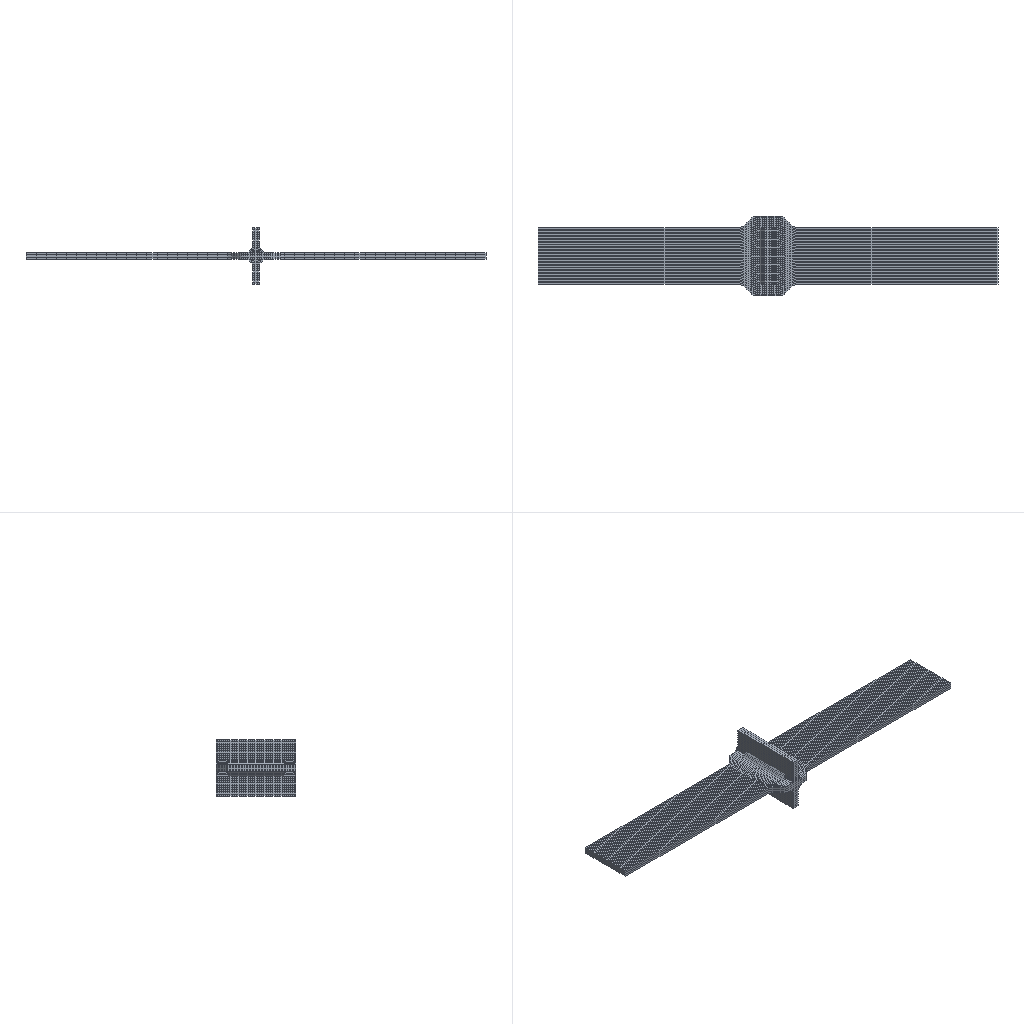Simulation study | abaqus
Set-up summary:
category,name,step,type,value,unit,region
solver,abaqus
solver,version,,,Abaqus/Standard 3DEXPERIENCE R2017x
units,not stated in the deck,,not stated
analysis,deck,,coupled temperature-displacement,coupled temperature-displacement
load_step,Step-del,Step-del,coupled temperature-displacement
load_step,Step-add,Step-add,coupled temperature-displacement
load_step,requested,,,2
mesh,nodes,,,15296
mesh,elements,,,11153
element_type,C3D8RT,,solid,11153
load,load commands in deck,,count,3
bc,support commands in deck,,count,3
material,MATERIAL-1,,in results
check,setup vs results,,match,"per instance, exact: element labels, types and connectivity; labels of the nodes the elements use; coordinates of those nodes at SINGLE_PRECISION in 1 of 2 instance(s)"
Abaqus input file, long lists of numbers shortened:
*Heading
** Job name: Job-2 Model name: Model-1-Copy
** Generated by: Abaqus/CAE 2017
*Preprint, echo=NO, model=NO, history=NO, contact=NO
**
** PARTS
**
*Part, name=Part-1
*Node
      1,  -10.243,          70.,           6.
      2,  -10.243,          70.,           0.
** (14566 more lines like these left out)
*Element, type=C3D8RT
1,  134, 1857,  129,    1,  135, 1859,  136,    6
2, 1857, 1858,  130,  129, 1859, 1860,  137,  136
** (10676 more lines like these left out)
*Nset, nset=Set-5, generate
     1,  14568,      1
*Elset, elset=Set-5, generate
     1,  10678,      1
** Section: Section-1
*Solid Section, elset=Set-5, material=Material-1
,
*End Part
**
*Part, name=add
*Node
      1,   4.243,          60.,           6.
      2,   4.243,          10.,           6.
** (726 more lines like these left out)
*Element, type=C3D8RT
  1, 273, 276,  96,  95, 441, 444, 299, 300
  2, 276, 275,  97,  96, 444, 443, 298, 299
** (473 more lines like these left out)
*Nset, nset=Set-5, generate
   1,  728,    1
*Elset, elset=Set-5, generate
   1,  475,    1
** Section: Section-1
*Solid Section, elset=Set-5, material=Material-1
,
*End Part
**
**
** ASSEMBLY
**
*Assembly, name=Assembly
**
*Instance, name=Part-1-1, part=Part-1
    -2.121,         -10.,     -8.121
*End Instance
**
*Instance, name=add-1, part=add
    -2.121,         -10.,     -8.121
*End Instance
**
*Nset, nset=Set-1, instance=Part-1-1
    13,    14,    15,    16,    33,    34,    44,    45,    49,    50,    54,    55,    65,    70,    71,    76
    82,    91,   213,   214,   215,   216,   217,   218,   219,   220,   221,   222,   223,   224,   225,   226
** (52 more lines like these left out)
*Elset, elset=Set-1, instance=Part-1-1, generate
 10213,  10637,      1
*Nset, nset=Set-4, instance=Part-1-1
    99,   100,   103,   104,   109,   110,   111,   112,   115,   116,   119,   120,   125,   126,   127,   128
  1024,  1025,  1026,  1027,  1028,  1029,  1030,  1031,  1032,  1033,  1034,  1035,  1036,  1037,  1038,  1039
** (397 more lines like these left out)
*Elset, elset=Set-4, instance=Part-1-1
 4108, 4109, 4110, 4111, 4112, 4113, 4114, 4115, 4116, 4117, 4118, 4119, 4120, 4121, 4122, 4123
 4124, 4125, 4126, 4127, 4128, 4129, 4130, 4131, 4132, 4133, 4134, 4135, 4136, 4137, 4138, 4139
** (276 more lines like these left out)
*Nset, nset=Set-5, instance=Part-1-1, generate
     1,  14568,      1
*Elset, elset=Set-5, instance=Part-1-1, generate
     1,  10678,      1
*Nset, nset=Set-6, instance=add-1, generate
   1,  728,    1
*Elset, elset=Set-6, instance=add-1, generate
   1,  475,    1
*Nset, nset=Set-7, instance=Part-1-1, generate
     1,  14568,      1
*Nset, nset=Set-7, instance=add-1, generate
   1,  728,    1
*Elset, elset=Set-7, instance=Part-1-1, generate
     1,  10678,      1
*Elset, elset=Set-7, instance=add-1, generate
   1,  475,    1
*Nset, nset=Set-8, instance=Part-1-1
    13,    14,    15,    16,    33,    34,    44,    45,    49,    50,    54,    55,    65,    70,    71,    76
    82,    91,   213,   214,   215,   216,   217,   218,   219,   220,   221,   222,   223,   224,   225,   226
** (52 more lines like these left out)
*Nset, nset=Set-8, instance=add-1, generate
   1,  728,    1
*Elset, elset=Set-8, instance=Part-1-1, generate
 10213,  10637,      1
*Elset, elset=Set-8, instance=add-1, generate
   1,  475,    1
*Nset, nset=Set-9, instance=add-1, generate
   1,  728,    1
*Elset, elset=Set-9, instance=add-1, generate
   1,  475,    1
*Nset, nset=Set-10, instance=Part-1-1, generate
     1,  14568,      1
*Nset, nset=Set-10, instance=add-1, generate
   1,  728,    1
*Elset, elset=Set-10, instance=Part-1-1, generate
     1,  10678,      1
*Elset, elset=Set-10, instance=add-1, generate
   1,  475,    1
*Elset, elset=_Surf-1_S4, internal, instance=Part-1-1
     3,     6,     9,    12,    15,    18,    21,    24,    27,    30,    33,    36,    39,    42,    45,    48
    51,    54,    57,    60,    63,    66,    69,    72,    75,    78,    81,    84,    87,    90,    93,    96
** (63 more lines like these left out)
*Elset, elset=_Surf-1_S6, internal, instance=Part-1-1
     1,     4,     7,    10,    13,    16,    19,    22,    25,    28,    31,    34,    37,    40,    43,    46
    49,    52,    55,    58,    61,    64,    67,    70,    73,    76,    79,    82,    85,    88,    91,    94
** (50 more lines like these left out)
*Elset, elset=_Surf-1_S3, internal, instance=Part-1-1
  445,  446,  447,  556,  557,  558,  667,  668,  669,  781,  784,  787,  790,  793,  871,  874
  877,  880,  883,  892,  895,  898,  901,  904,  982,  985,  988,  991,  994, 1003, 1006, 1009
** (38 more lines like these left out)
*Elset, elset=_Surf-1_S5, internal, instance=Part-1-1
   553,   554,   555,   664,   665,   666,   775,   776,   777,   783,   786,   789,   792,   795,   873,   876
   879,   882,   885,   894,   897,   900,   903,   906,   984,   987,   990,   993,   996,  1005,  1008,  1011
** (31 more lines like these left out)
*Elset, elset=_Surf-1_S1, internal, instance=Part-1-1
     1,     2,     3,     4,     5,     6,   223,   224,   225,   226,   227,   228,  3553,  3554,  3555,  3556
  3557,  3558,  3559,  3560,  3561,  3562,  3563,  3564,  3565,  3566,  3567,  3568,  3569,  3570,  3571,  3572
** (133 more lines like these left out)
*Elset, elset=_Surf-1_S2, internal, instance=Part-1-1
   217,   218,   219,   220,   221,   222,   439,   440,   441,   442,   443,   444,  1999,  2000,  2001,  2002
  2003,  2004,  2005,  2006,  2007,  2008,  2009,  2010,  2011,  2012,  2013,  2014,  2015,  2016,  2017,  2018
** (147 more lines like these left out)
*Surface, type=ELEMENT, name=Surf-1
_Surf-1_S4, S4
_Surf-1_S6, S6
_Surf-1_S2, S2
_Surf-1_S3, S3
_Surf-1_S5, S5
_Surf-1_S1, S1
*Elset, elset=_Surf-2_S4, internal, instance=Part-1-1
     3,     6,     9,    12,    15,    18,    21,    24,    27,    30,    33,    36,    39,    42,    45,    48
    51,    54,    57,    60,    63,    66,    69,    72,    75,    78,    81,    84,    87,    90,    93,    96
** (63 more lines like these left out)
*Elset, elset=_Surf-2_S6, internal, instance=Part-1-1
     1,     4,     7,    10,    13,    16,    19,    22,    25,    28,    31,    34,    37,    40,    43,    46
    49,    52,    55,    58,    61,    64,    67,    70,    73,    76,    79,    82,    85,    88,    91,    94
** (50 more lines like these left out)
*Elset, elset=_Surf-2_S3, internal, instance=Part-1-1
  445,  446,  447,  556,  557,  558,  667,  668,  669,  781,  784,  787,  790,  793,  871,  874
  877,  880,  883,  892,  895,  898,  901,  904,  982,  985,  988,  991,  994, 1003, 1006, 1009
** (38 more lines like these left out)
*Elset, elset=_Surf-2_S5, internal, instance=Part-1-1
   553,   554,   555,   664,   665,   666,   775,   776,   777,   783,   786,   789,   792,   795,   873,   876
   879,   882,   885,   894,   897,   900,   903,   906,   984,   987,   990,   993,   996,  1005,  1008,  1011
** (31 more lines like these left out)
*Elset, elset=_Surf-2_S1, internal, instance=Part-1-1
     1,     2,     3,     4,     5,     6,   223,   224,   225,   226,   227,   228,  3553,  3554,  3555,  3556
  3557,  3558,  3559,  3560,  3561,  3562,  3563,  3564,  3565,  3566,  3567,  3568,  3569,  3570,  3571,  3572
** (133 more lines like these left out)
*Elset, elset=_Surf-2_S2, internal, instance=Part-1-1
   217,   218,   219,   220,   221,   222,   439,   440,   441,   442,   443,   444,  1999,  2000,  2001,  2002
  2003,  2004,  2005,  2006,  2007,  2008,  2009,  2010,  2011,  2012,  2013,  2014,  2015,  2016,  2017,  2018
** (147 more lines like these left out)
*Surface, type=ELEMENT, name=Surf-2
_Surf-2_S4, S4
_Surf-2_S6, S6
_Surf-2_S2, S2
_Surf-2_S3, S3
_Surf-2_S5, S5
_Surf-2_S1, S1
*Elset, elset=_Surf-5_S4, internal, instance=Part-1-1
     3,     6,     9,    12,    15,    18,    21,    24,    27,    30,    33,    36,    39,    42,    45,    48
    51,    54,    57,    60,    63,    66,    69,    72,    75,    78,    81,    84,    87,    90,    93,    96
** (63 more lines like these left out)
*Elset, elset=_Surf-5_S4, internal, instance=add-1
   4,   7,  10,  13,  16,  17,  18,  19,  23,  26,  29,  32,  35,  36,  37,  38
  42,  45,  48,  51,  54,  55,  56,  57,  61,  64,  67,  70,  73,  74,  75,  76
** (11 more lines like these left out)
*Elset, elset=_Surf-5_S6, internal, instance=Part-1-1
     1,     4,     7,    10,    13,    16,    19,    22,    25,    28,    31,    34,    37,    40,    43,    46
    49,    52,    55,    58,    61,    64,    67,    70,    73,    76,    79,    82,    85,    88,    91,    94
** (50 more lines like these left out)
*Elset, elset=_Surf-5_S3, internal, instance=Part-1-1
  445,  446,  447,  556,  557,  558,  667,  668,  669,  781,  784,  787,  790,  793,  871,  874
  877,  880,  883,  892,  895,  898,  901,  904,  982,  985,  988,  991,  994, 1003, 1006, 1009
** (38 more lines like these left out)
*Elset, elset=_Surf-5_S5, internal, instance=Part-1-1
   553,   554,   555,   664,   665,   666,   775,   776,   777,   783,   786,   789,   792,   795,   873,   876
   879,   882,   885,   894,   897,   900,   903,   906,   984,   987,   990,   993,   996,  1005,  1008,  1011
** (31 more lines like these left out)
*Elset, elset=_Surf-5_S5, internal, instance=add-1
   1,   2,   3,   4,   5,   6,   7,  17,  20,  21,  22,  23,  24,  25,  26,  36
  39,  40,  41,  42,  43,  44,  45,  55,  58,  59,  60,  61,  62,  63,  64,  74
** (11 more lines like these left out)
*Elset, elset=_Surf-5_S1, internal, instance=Part-1-1
     1,     2,     3,     4,     5,     6,   223,   224,   225,   226,   227,   228,  3553,  3554,  3555,  3556
  3557,  3558,  3559,  3560,  3561,  3562,  3563,  3564,  3565,  3566,  3567,  3568,  3569,  3570,  3571,  3572
** (133 more lines like these left out)
*Elset, elset=_Surf-5_S1, internal, instance=add-1, generate
  1,  19,   1
*Elset, elset=_Surf-5_S2, internal, instance=Part-1-1
   217,   218,   219,   220,   221,   222,   439,   440,   441,   442,   443,   444,  1999,  2000,  2001,  2002
  2003,  2004,  2005,  2006,  2007,  2008,  2009,  2010,  2011,  2012,  2013,  2014,  2015,  2016,  2017,  2018
** (147 more lines like these left out)
*Elset, elset=_Surf-5_S2, internal, instance=add-1, generate
 457,  475,    1
*Surface, type=ELEMENT, name=Surf-5
_Surf-5_S4, S4
_Surf-5_S6, S6
_Surf-5_S2, S2
_Surf-5_S3, S3
_Surf-5_S5, S5
_Surf-5_S1, S1
*Elset, elset=_Surf-6_S4, internal, instance=Part-1-1
     3,     6,     9,    12,    15,    18,    21,    24,    27,    30,    33,    36,    39,    42,    45,    48
    51,    54,    57,    60,    63,    66,    69,    72,    75,    78,    81,    84,    87,    90,    93,    96
** (63 more lines like these left out)
*Elset, elset=_Surf-6_S4, internal, instance=add-1
   4,   7,  10,  13,  16,  17,  18,  19,  23,  26,  29,  32,  35,  36,  37,  38
  42,  45,  48,  51,  54,  55,  56,  57,  61,  64,  67,  70,  73,  74,  75,  76
** (11 more lines like these left out)
*Elset, elset=_Surf-6_S6, internal, instance=Part-1-1
     1,     4,     7,    10,    13,    16,    19,    22,    25,    28,    31,    34,    37,    40,    43,    46
    49,    52,    55,    58,    61,    64,    67,    70,    73,    76,    79,    82,    85,    88,    91,    94
** (50 more lines like these left out)
*Elset, elset=_Surf-6_S3, internal, instance=Part-1-1
  445,  446,  447,  556,  557,  558,  667,  668,  669,  781,  784,  787,  790,  793,  871,  874
  877,  880,  883,  892,  895,  898,  901,  904,  982,  985,  988,  991,  994, 1003, 1006, 1009
** (38 more lines like these left out)
*Elset, elset=_Surf-6_S5, internal, instance=Part-1-1
   553,   554,   555,   664,   665,   666,   775,   776,   777,   783,   786,   789,   792,   795,   873,   876
   879,   882,   885,   894,   897,   900,   903,   906,   984,   987,   990,   993,   996,  1005,  1008,  1011
** (31 more lines like these left out)
*Elset, elset=_Surf-6_S5, internal, instance=add-1
   1,   2,   3,   4,   5,   6,   7,  17,  20,  21,  22,  23,  24,  25,  26,  36
  39,  40,  41,  42,  43,  44,  45,  55,  58,  59,  60,  61,  62,  63,  64,  74
** (11 more lines like these left out)
*Elset, elset=_Surf-6_S1, internal, instance=Part-1-1
     1,     2,     3,     4,     5,     6,   223,   224,   225,   226,   227,   228,  3553,  3554,  3555,  3556
  3557,  3558,  3559,  3560,  3561,  3562,  3563,  3564,  3565,  3566,  3567,  3568,  3569,  3570,  3571,  3572
** (133 more lines like these left out)
*Elset, elset=_Surf-6_S1, internal, instance=add-1, generate
  1,  19,   1
*Elset, elset=_Surf-6_S2, internal, instance=Part-1-1
   217,   218,   219,   220,   221,   222,   439,   440,   441,   442,   443,   444,  1999,  2000,  2001,  2002
  2003,  2004,  2005,  2006,  2007,  2008,  2009,  2010,  2011,  2012,  2013,  2014,  2015,  2016,  2017,  2018
** (147 more lines like these left out)
*Elset, elset=_Surf-6_S2, internal, instance=add-1, generate
 457,  475,    1
*Surface, type=ELEMENT, name=Surf-6
_Surf-6_S4, S4
_Surf-6_S6, S6
_Surf-6_S2, S2
_Surf-6_S3, S3
_Surf-6_S5, S5
_Surf-6_S1, S1
*Elset, elset=_m_Surf-3_S4, internal, instance=add-1
   4,   7,  10,  13,  16,  23,  26,  29,  32,  35,  42,  45,  48,  51,  54,  61
  64,  67,  70,  73,  80,  83,  86,  89,  92,  99, 102, 105, 108, 111, 118, 121
** (6 more lines like these left out)
*Elset, elset=_m_Surf-3_S5, internal, instance=add-1
   5,   6,   7,  17,  24,  25,  26,  36,  43,  44,  45,  55,  62,  63,  64,  74
  81,  82,  83,  93, 100, 101, 102, 112, 119, 120, 121, 131, 138, 139, 140, 150
** (5 more lines like these left out)
*Surface, type=ELEMENT, name=m_Surf-3
_m_Surf-3_S4, S4
_m_Surf-3_S5, S5
*Elset, elset=_s_Surf-3_S4, internal, instance=Part-1-1
 2115, 2118, 2121, 2124, 2127, 2130, 2133, 2136, 2139, 2142, 2145, 2148, 2151, 2154, 2157, 2160
 2163, 2166, 2169, 2172, 2175, 2178, 2181, 2184, 2187, 2190, 2193, 2196, 2199, 2202, 2205, 2208
** (7 more lines like these left out)
*Elset, elset=_s_Surf-3_S6, internal, instance=Part-1-1, generate
 3886,  4099,     3
*Surface, type=ELEMENT, name=s_Surf-3
_s_Surf-3_S4, S4
_s_Surf-3_S6, S6
** Constraint: Constraint-1
*Tie, name=Constraint-1, adjust=yes
m_Surf-3, s_Surf-3
*End Assembly
**
** MATERIALS
**
*Material, name=Material-1
*Conductivity
45.,
*Density
 7.8e-09,
*Elastic
210000., 0.3
*Expansion
 1.2e-05,
*Plastic
350.,0.
*Specific Heat
 4.6e+08,
**
** PHYSICAL CONSTANTS
**
*Physical Constants, absolute zero=-273., stefan boltzmann=5.67e-08
**
** PREDEFINED FIELDS
**
** Name: Predefined Field-1   Type: Temperature
*Initial Conditions, type=TEMPERATURE
Set-7, 20.
** ----------------------------------------------------------------
**
** STEP: Step-del
**
*Step, name=Step-del, nlgeom=NO
*Coupled Temperature-displacement, creep=none, deltmx=1e+12, stabilize=0.0002, allsdtol=0.05, continue=NO
0.0001, 0.0001, 1e-09, 0.0001
**
** BOUNDARY CONDITIONS
**
** Name: BC-1 Type: 对称/反对称/完全固定
*Boundary
Set-4, ENCASTRE
**
** INTERACTIONS
**
** Interaction: Int-del
*Model Change, remove
Set-8,
**
** OUTPUT REQUESTS
**
*Restart, write, frequency=0
**
** FIELD OUTPUT: F-Output-1
**
*Output, field
*Node Output
CF, NT, RF, RFL, RM, RT, U, V
*Element Output, directions=YES
E, HFL, LE, MISES, MISESMAX, MISESONLY, PE, PEEQ, PEEQMAX, PEEQT, PEMAG, S, SSAVG, TEMP
*Contact Output
CDISP, CSTRESS
*Radiation Output
FTEMP,
**
** HISTORY OUTPUT: H-Output-1
**
*Output, history, variable=PRESELECT
*End Step
** ----------------------------------------------------------------
**
** STEP: Step-add
**
*Step, name=Step-add, nlgeom=YES, inc=10000000
*Coupled Temperature-displacement, creep=none, deltmx=1e+12
0.05, 10., 1e-06, 0.5
**
** LOADS
**
** Name: Load-1   Type: Body heat flux
*Dflux
Set-10, BFNU, 1.
**
** INTERACTIONS
**
** Interaction: Int-add
*Model Change, add
Set-9,
** Interaction: Int-3
*Sradiate
Surf-5, R, 20., 0.5
** Interaction: Int-4
*Sfilm
Surf-6, F, 20., 0.0002
**
** OUTPUT REQUESTS
**
*Restart, write, frequency=0
**
** FIELD OUTPUT: F-Output-1
**
*Output, field
*Node Output
CF, NT, RF, RFL, RM, RT, U, V
*Element Output, directions=YES
E, HFL, LE, MISES, MISESMAX, MISESONLY, PE, PEEQ, PEEQMAX, PEEQT, PEMAG, S, SSAVG, TEMP
*Contact Output
CDISP, CSTRESS
*Radiation Output
FTEMP,
**
** HISTORY OUTPUT: H-Output-1
**
*Output, history, variable=PRESELECT
*End Step
Results summary:
result,step,,completed,increments=1 time=0.0001/0.0001
result,step,,completed,increments=69 time=10.0/10.0
result,analysis,,,"coupled temperature-displacement, steady state"
result,last_loadstep,,,2
result,primary field,,,"U, NT11"
result,reaction total,,FX,-6e-06,model units
result,reaction total,,FY,9e-06,model units
result,reaction total,,FZ,-1e-05,model units